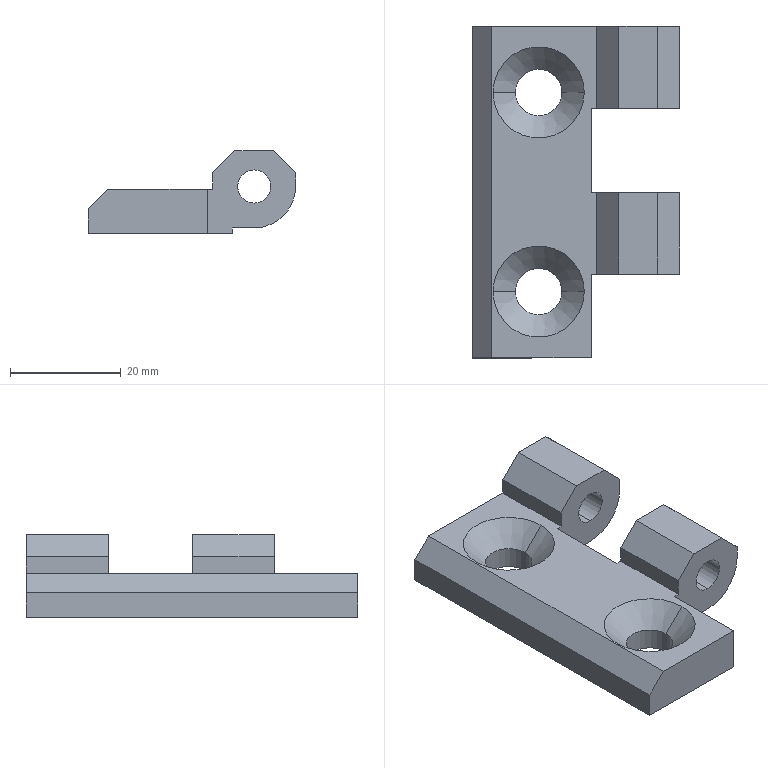Part | SolidWorks | features BaseBody 1 | 1 solid | 39 faces | box 37.5 x 60 x 15 mm | volume 13374 mm3 | plane 25 | cylinder 10 | cone 4 | commonest cylinder face diameters 6 x4 8.4 x4 15 x2
STEP:
#1=CARTESIAN_POINT('',(-13.8,-18.,0.));
#2=VERTEX_POINT('',#1);
#3=CARTESIAN_POINT('',(-22.2,-18.,0.));
#4=VERTEX_POINT('',#3);
#5=CARTESIAN_POINT('',(-18.,-18.,0.));
#6=DIRECTION('',(0.,0.,-1.));
#7=DIRECTION('',(1.,0.,0.));
#8=AXIS2_PLACEMENT_3D('',#5,#6,#7);
#9=CIRCLE('',#8,4.2);
#10=EDGE_CURVE('',#2,#4,#9,.T.);
#11=ORIENTED_EDGE('',*,*,#10,.T.);
#12=CARTESIAN_POINT('',(-22.2,-18.,3.95));
#13=VERTEX_POINT('',#12);
#14=CARTESIAN_POINT('',(-22.2,-18.,0.));
#15=DIRECTION('',(0.,0.,1.));
#16=VECTOR('',#15,1000.);
#17=LINE('',#14,#16);
#18=EDGE_CURVE('',#4,#13,#17,.T.);
#19=ORIENTED_EDGE('',*,*,#18,.T.);
#20=CARTESIAN_POINT('',(-13.8,-18.,3.95));
#21=VERTEX_POINT('',#20);
#22=CARTESIAN_POINT('',(-18.,-18.,3.95));
#23=DIRECTION('',(0.,0.,-1.));
#24=DIRECTION('',(1.,0.,0.));
#25=AXIS2_PLACEMENT_3D('',#22,#23,#24);
#26=CIRCLE('',#25,4.2);
#27=EDGE_CURVE('',#21,#13,#26,.T.);
#28=ORIENTED_EDGE('',*,*,#27,.F.);
#29=CARTESIAN_POINT('',(-13.8,-18.,0.));
#30=DIRECTION('',(0.,0.,1.));
#31=VECTOR('',#30,1000.);
#32=LINE('',#29,#31);
#33=EDGE_CURVE('',#2,#21,#32,.T.);
#34=ORIENTED_EDGE('',*,*,#33,.F.);
#35=EDGE_LOOP('',(#11,#19,#28,#34));
#36=FACE_OUTER_BOUND('',#35,.T.);
#37=CARTESIAN_POINT('',(-18.,-18.,0.));
#38=DIRECTION('',(0.,0.,1.));
#39=DIRECTION('',(1.,0.,0.));
#40=AXIS2_PLACEMENT_3D('',#37,#38,#39);
#41=CYLINDRICAL_SURFACE('',#40,4.2);
#42=ADVANCED_FACE('',(#36),#41,.F.);
#43=CARTESIAN_POINT('',(-13.8,18.,0.));
#44=VERTEX_POINT('',#43);
#45=CARTESIAN_POINT('',(-22.2,18.,0.));
#46=VERTEX_POINT('',#45);
#47=CARTESIAN_POINT('',(-18.,18.,0.));
#48=DIRECTION('',(0.,0.,-1.));
#49=DIRECTION('',(1.,0.,0.));
#50=AXIS2_PLACEMENT_3D('',#47,#48,#49);
#51=CIRCLE('',#50,4.2);
#52=EDGE_CURVE('',#44,#46,#51,.T.);
#53=ORIENTED_EDGE('',*,*,#52,.T.);
#54=CARTESIAN_POINT('',(-22.2,18.,3.95));
#55=VERTEX_POINT('',#54);
#56=CARTESIAN_POINT('',(-22.2,18.,0.));
#57=DIRECTION('',(0.,0.,1.));
#58=VECTOR('',#57,1000.);
#59=LINE('',#56,#58);
#60=EDGE_CURVE('',#46,#55,#59,.T.);
#61=ORIENTED_EDGE('',*,*,#60,.T.);
#62=CARTESIAN_POINT('',(-13.8,18.,3.95));
#63=VERTEX_POINT('',#62);
#64=CARTESIAN_POINT('',(-18.,18.,3.95));
#65=DIRECTION('',(0.,0.,-1.));
#66=DIRECTION('',(1.,0.,0.));
#67=AXIS2_PLACEMENT_3D('',#64,#65,#66);
#68=CIRCLE('',#67,4.2);
#69=EDGE_CURVE('',#63,#55,#68,.T.);
#70=ORIENTED_EDGE('',*,*,#69,.F.);
#71=CARTESIAN_POINT('',(-13.8,18.,0.));
#72=DIRECTION('',(0.,0.,1.));
#73=VECTOR('',#72,1000.);
#74=LINE('',#71,#73);
#75=EDGE_CURVE('',#44,#63,#74,.T.);
#76=ORIENTED_EDGE('',*,*,#75,.F.);
#77=EDGE_LOOP('',(#53,#61,#70,#76));
#78=FACE_OUTER_BOUND('',#77,.T.);
#79=CARTESIAN_POINT('',(-18.,18.,0.));
#80=DIRECTION('',(0.,0.,1.));
#81=DIRECTION('',(1.,0.,0.));
#82=AXIS2_PLACEMENT_3D('',#79,#80,#81);
#83=CYLINDRICAL_SURFACE('',#82,4.2);
#84=ADVANCED_FACE('',(#78),#83,.F.);
#85=ORIENTED_EDGE('',*,*,#27,.T.);
#86=CARTESIAN_POINT('',(-26.25,-18.,8.));
#87=VERTEX_POINT('',#86);
#88=CARTESIAN_POINT('',(-26.25,-18.,8.));
#89=DIRECTION('',(-0.7071,0.,0.7071));
#90=VECTOR('',#89,1000.);
#91=LINE('',#88,#90);
#92=EDGE_CURVE('',#13,#87,#91,.T.);
#93=ORIENTED_EDGE('',*,*,#92,.T.);
#94=CARTESIAN_POINT('',(-9.75,-18.,8.));
#95=VERTEX_POINT('',#94);
#96=CARTESIAN_POINT('',(-18.,-18.,8.));
#97=DIRECTION('',(0.,0.,-1.));
#98=DIRECTION('',(1.,0.,0.));
#99=AXIS2_PLACEMENT_3D('',#96,#97,#98);
#100=CIRCLE('',#99,8.25);
#101=EDGE_CURVE('',#95,#87,#100,.T.);
#102=ORIENTED_EDGE('',*,*,#101,.F.);
#103=CARTESIAN_POINT('',(-9.75,-18.,8.));
#104=DIRECTION('',(0.7071,0.,0.7071));
#105=VECTOR('',#104,1000.);
#106=LINE('',#103,#105);
#107=EDGE_CURVE('',#21,#95,#106,.T.);
#108=ORIENTED_EDGE('',*,*,#107,.F.);
#109=EDGE_LOOP('',(#85,#93,#102,#108));
#110=FACE_OUTER_BOUND('',#109,.T.);
#111=CARTESIAN_POINT('',(-18.,-18.,8.));
#112=DIRECTION('',(0.,0.,1.));
#113=DIRECTION('',(1.,0.,0.));
#114=AXIS2_PLACEMENT_3D('',#111,#112,#113);
#115=CONICAL_SURFACE('',#114,8.25,0.7854);
#116=ADVANCED_FACE('',(#110),#115,.F.);
#117=ORIENTED_EDGE('',*,*,#69,.T.);
#118=CARTESIAN_POINT('',(-26.25,18.,8.));
#119=VERTEX_POINT('',#118);
#120=CARTESIAN_POINT('',(-26.25,18.,8.));
#121=DIRECTION('',(-0.7071,0.,0.7071));
#122=VECTOR('',#121,1000.);
#123=LINE('',#120,#122);
#124=EDGE_CURVE('',#55,#119,#123,.T.);
#125=ORIENTED_EDGE('',*,*,#124,.T.);
#126=CARTESIAN_POINT('',(-9.75,18.,8.));
#127=VERTEX_POINT('',#126);
#128=CARTESIAN_POINT('',(-18.,18.,8.));
#129=DIRECTION('',(0.,0.,-1.));
#130=DIRECTION('',(1.,0.,0.));
#131=AXIS2_PLACEMENT_3D('',#128,#129,#130);
#132=CIRCLE('',#131,8.25);
#133=EDGE_CURVE('',#127,#119,#132,.T.);
#134=ORIENTED_EDGE('',*,*,#133,.F.);
#135=CARTESIAN_POINT('',(-9.75,18.,8.));
#136=DIRECTION('',(0.7071,0.,0.7071));
#137=VECTOR('',#136,1000.);
#138=LINE('',#135,#137);
#139=EDGE_CURVE('',#63,#127,#138,.T.);
#140=ORIENTED_EDGE('',*,*,#139,.F.);
#141=EDGE_LOOP('',(#117,#125,#134,#140));
#142=FACE_OUTER_BOUND('',#141,.T.);
#143=CARTESIAN_POINT('',(-18.,18.,8.));
#144=DIRECTION('',(0.,0.,1.));
#145=DIRECTION('',(1.,0.,0.));
#146=AXIS2_PLACEMENT_3D('',#143,#144,#145);
#147=CONICAL_SURFACE('',#146,8.25,0.7854);
#148=ADVANCED_FACE('',(#142),#147,.F.);
#149=CARTESIAN_POINT('',(0.,-14.85,5.5));
#150=VERTEX_POINT('',#149);
#151=CARTESIAN_POINT('',(0.,-14.85,11.5));
#152=VERTEX_POINT('',#151);
#153=CARTESIAN_POINT('',(0.,-14.85,8.5));
#154=DIRECTION('',(0.,1.,0.));
#155=DIRECTION('',(0.,0.,1.));
#156=AXIS2_PLACEMENT_3D('',#153,#154,#155);
#157=CIRCLE('',#156,3.);
#158=EDGE_CURVE('',#150,#152,#157,.T.);
#159=ORIENTED_EDGE('',*,*,#158,.F.);
#160=CARTESIAN_POINT('',(0.,-0.15,5.5));
#161=VERTEX_POINT('',#160);
#162=CARTESIAN_POINT('',(0.,-30.,5.5));
#163=DIRECTION('',(0.,1.,0.));
#164=VECTOR('',#163,1000.);
#165=LINE('',#162,#164);
#166=EDGE_CURVE('',#150,#161,#165,.T.);
#167=ORIENTED_EDGE('',*,*,#166,.T.);
#168=CARTESIAN_POINT('',(0.,-0.15,11.5));
#169=VERTEX_POINT('',#168);
#170=CARTESIAN_POINT('',(0.,-0.15,8.5));
#171=DIRECTION('',(0.,-1.,0.));
#172=DIRECTION('',(0.,0.,1.));
#173=AXIS2_PLACEMENT_3D('',#170,#171,#172);
#174=CIRCLE('',#173,3.);
#175=EDGE_CURVE('',#169,#161,#174,.T.);
#176=ORIENTED_EDGE('',*,*,#175,.F.);
#177=CARTESIAN_POINT('',(0.,-30.,11.5));
#178=DIRECTION('',(0.,1.,0.));
#179=VECTOR('',#178,1000.);
#180=LINE('',#177,#179);
#181=EDGE_CURVE('',#152,#169,#180,.T.);
#182=ORIENTED_EDGE('',*,*,#181,.F.);
#183=EDGE_LOOP('',(#159,#167,#176,#182));
#184=FACE_OUTER_BOUND('',#183,.T.);
#185=CARTESIAN_POINT('',(0.,-30.,8.5));
#186=DIRECTION('',(0.,1.,0.));
#187=DIRECTION('',(0.,0.,1.));
#188=AXIS2_PLACEMENT_3D('',#185,#186,#187);
#189=CYLINDRICAL_SURFACE('',#188,3.);
#190=ADVANCED_FACE('',(#184),#189,.F.);
#191=CARTESIAN_POINT('',(0.,15.15,5.5));
#192=VERTEX_POINT('',#191);
#193=CARTESIAN_POINT('',(0.,15.15,11.5));
#194=VERTEX_POINT('',#193);
#195=CARTESIAN_POINT('',(0.,15.15,8.5));
#196=DIRECTION('',(0.,1.,0.));
#197=DIRECTION('',(0.,0.,1.));
#198=AXIS2_PLACEMENT_3D('',#195,#196,#197);
#199=CIRCLE('',#198,3.);
#200=EDGE_CURVE('',#192,#194,#199,.T.);
#201=ORIENTED_EDGE('',*,*,#200,.F.);
#202=CARTESIAN_POINT('',(0.,30.,5.5));
#203=VERTEX_POINT('',#202);
#204=CARTESIAN_POINT('',(0.,-30.,5.5));
#205=DIRECTION('',(0.,1.,0.));
#206=VECTOR('',#205,1000.);
#207=LINE('',#204,#206);
#208=EDGE_CURVE('',#192,#203,#207,.T.);
#209=ORIENTED_EDGE('',*,*,#208,.T.);
#210=CARTESIAN_POINT('',(0.,30.,11.5));
#211=VERTEX_POINT('',#210);
#212=CARTESIAN_POINT('',(0.,30.,8.5));
#213=DIRECTION('',(0.,-1.,0.));
#214=DIRECTION('',(0.,0.,1.));
#215=AXIS2_PLACEMENT_3D('',#212,#213,#214);
#216=CIRCLE('',#215,3.);
#217=EDGE_CURVE('',#211,#203,#216,.T.);
#218=ORIENTED_EDGE('',*,*,#217,.F.);
#219=CARTESIAN_POINT('',(0.,-30.,11.5));
#220=DIRECTION('',(0.,1.,0.));
#221=VECTOR('',#220,1000.);
#222=LINE('',#219,#221);
#223=EDGE_CURVE('',#194,#211,#222,.T.);
#224=ORIENTED_EDGE('',*,*,#223,.F.);
#225=EDGE_LOOP('',(#201,#209,#218,#224));
#226=FACE_OUTER_BOUND('',#225,.T.);
#227=CARTESIAN_POINT('',(0.,-30.,8.5));
#228=DIRECTION('',(0.,1.,0.));
#229=DIRECTION('',(0.,0.,1.));
#230=AXIS2_PLACEMENT_3D('',#227,#228,#229);
#231=CYLINDRICAL_SURFACE('',#230,3.);
#232=ADVANCED_FACE('',(#226),#231,.F.);
#233=ORIENTED_EDGE('',*,*,#10,.F.);
#234=CARTESIAN_POINT('',(-18.,-18.,0.));
#235=DIRECTION('',(0.,0.,-1.));
#236=DIRECTION('',(1.,0.,0.));
#237=AXIS2_PLACEMENT_3D('',#234,#235,#236);
#238=CIRCLE('',#237,4.2);
#239=EDGE_CURVE('',#4,#2,#238,.T.);
#240=ORIENTED_EDGE('',*,*,#239,.F.);
#241=EDGE_LOOP('',(#233,#240));
#242=FACE_BOUND('',#241,.T.);
#243=ORIENTED_EDGE('',*,*,#52,.F.);
#244=CARTESIAN_POINT('',(-18.,18.,0.));
#245=DIRECTION('',(0.,0.,-1.));
#246=DIRECTION('',(1.,0.,0.));
#247=AXIS2_PLACEMENT_3D('',#244,#245,#246);
#248=CIRCLE('',#247,4.2);
#249=EDGE_CURVE('',#46,#44,#248,.T.);
#250=ORIENTED_EDGE('',*,*,#249,.F.);
#251=EDGE_LOOP('',(#243,#250));
#252=FACE_BOUND('',#251,.T.);
#253=CARTESIAN_POINT('',(-8.5,-14.85,0.));
#254=VERTEX_POINT('',#253);
#255=CARTESIAN_POINT('',(-4.,-14.85,0.));
#256=VERTEX_POINT('',#255);
#257=CARTESIAN_POINT('',(-4.,-14.85,0.));
#258=DIRECTION('',(1.,0.,0.));
#259=VECTOR('',#258,1000.);
#260=LINE('',#257,#259);
#261=EDGE_CURVE('',#254,#256,#260,.T.);
#262=ORIENTED_EDGE('',*,*,#261,.F.);
#263=CARTESIAN_POINT('',(-8.5,-30.,0.));
#264=VERTEX_POINT('',#263);
#265=CARTESIAN_POINT('',(-8.5,30.,0.));
#266=DIRECTION('',(0.,1.,0.));
#267=VECTOR('',#266,1000.);
#268=LINE('',#265,#267);
#269=EDGE_CURVE('',#264,#254,#268,.T.);
#270=ORIENTED_EDGE('',*,*,#269,.F.);
#271=CARTESIAN_POINT('',(-30.,-30.,0.));
#272=VERTEX_POINT('',#271);
#273=CARTESIAN_POINT('',(-4.,-30.,0.));
#274=DIRECTION('',(1.,0.,0.));
#275=VECTOR('',#274,1000.);
#276=LINE('',#273,#275);
#277=EDGE_CURVE('',#272,#264,#276,.T.);
#278=ORIENTED_EDGE('',*,*,#277,.F.);
#279=CARTESIAN_POINT('',(-30.,30.,0.));
#280=VERTEX_POINT('',#279);
#281=CARTESIAN_POINT('',(-30.,30.,0.));
#282=DIRECTION('',(0.,-1.,0.));
#283=VECTOR('',#282,1000.);
#284=LINE('',#281,#283);
#285=EDGE_CURVE('',#280,#272,#284,.T.);
#286=ORIENTED_EDGE('',*,*,#285,.F.);
#287=CARTESIAN_POINT('',(-4.,30.,0.));
#288=VERTEX_POINT('',#287);
#289=CARTESIAN_POINT('',(-4.,30.,0.));
#290=DIRECTION('',(-1.,0.,0.));
#291=VECTOR('',#290,1000.);
#292=LINE('',#289,#291);
#293=EDGE_CURVE('',#288,#280,#292,.T.);
#294=ORIENTED_EDGE('',*,*,#293,.F.);
#295=CARTESIAN_POINT('',(-4.,15.15,0.));
#296=VERTEX_POINT('',#295);
#297=CARTESIAN_POINT('',(-4.,30.,0.));
#298=DIRECTION('',(0.,1.,0.));
#299=VECTOR('',#298,1000.);
#300=LINE('',#297,#299);
#301=EDGE_CURVE('',#296,#288,#300,.T.);
#302=ORIENTED_EDGE('',*,*,#301,.F.);
#303=CARTESIAN_POINT('',(-8.5,15.15,0.));
#304=VERTEX_POINT('',#303);
#305=CARTESIAN_POINT('',(-4.,15.15,0.));
#306=DIRECTION('',(1.,0.,0.));
#307=VECTOR('',#306,1000.);
#308=LINE('',#305,#307);
#309=EDGE_CURVE('',#304,#296,#308,.T.);
#310=ORIENTED_EDGE('',*,*,#309,.F.);
#311=CARTESIAN_POINT('',(-8.5,-0.15,0.));
#312=VERTEX_POINT('',#311);
#313=CARTESIAN_POINT('',(-8.5,30.,0.));
#314=DIRECTION('',(0.,1.,0.));
#315=VECTOR('',#314,1000.);
#316=LINE('',#313,#315);
#317=EDGE_CURVE('',#312,#304,#316,.T.);
#318=ORIENTED_EDGE('',*,*,#317,.F.);
#319=CARTESIAN_POINT('',(-4.,-0.15,0.));
#320=VERTEX_POINT('',#319);
#321=CARTESIAN_POINT('',(-4.,-0.15,0.));
#322=DIRECTION('',(-1.,0.,0.));
#323=VECTOR('',#322,1000.);
#324=LINE('',#321,#323);
#325=EDGE_CURVE('',#320,#312,#324,.T.);
#326=ORIENTED_EDGE('',*,*,#325,.F.);
#327=CARTESIAN_POINT('',(-4.,30.,0.));
#328=DIRECTION('',(0.,1.,0.));
#329=VECTOR('',#328,1000.);
#330=LINE('',#327,#329);
#331=EDGE_CURVE('',#256,#320,#330,.T.);
#332=ORIENTED_EDGE('',*,*,#331,.F.);
#333=EDGE_LOOP('',(#262,#270,#278,#286,#294,#302,#310,#318,#326,#332));
#334=FACE_OUTER_BOUND('',#333,.T.);
#335=CARTESIAN_POINT('',(-4.,30.,0.));
#336=DIRECTION('',(0.,0.,1.));
#337=DIRECTION('',(1.,0.,0.));
#338=AXIS2_PLACEMENT_3D('',#335,#336,#337);
#339=PLANE('',#338);
#340=ADVANCED_FACE('',(#242,#252,#334),#339,.F.);
#341=ORIENTED_EDGE('',*,*,#18,.F.);
#342=ORIENTED_EDGE('',*,*,#239,.T.);
#343=ORIENTED_EDGE('',*,*,#33,.T.);
#344=CARTESIAN_POINT('',(-18.,-18.,3.95));
#345=DIRECTION('',(0.,0.,-1.));
#346=DIRECTION('',(1.,0.,0.));
#347=AXIS2_PLACEMENT_3D('',#344,#345,#346);
#348=CIRCLE('',#347,4.2);
#349=EDGE_CURVE('',#13,#21,#348,.T.);
#350=ORIENTED_EDGE('',*,*,#349,.F.);
#351=EDGE_LOOP('',(#341,#342,#343,#350));
#352=FACE_OUTER_BOUND('',#351,.T.);
#353=CARTESIAN_POINT('',(-18.,-18.,0.));
#354=DIRECTION('',(0.,0.,1.));
#355=DIRECTION('',(1.,0.,0.));
#356=AXIS2_PLACEMENT_3D('',#353,#354,#355);
#357=CYLINDRICAL_SURFACE('',#356,4.2);
#358=ADVANCED_FACE('',(#352),#357,.F.);
#359=ORIENTED_EDGE('',*,*,#60,.F.);
#360=ORIENTED_EDGE('',*,*,#249,.T.);
#361=ORIENTED_EDGE('',*,*,#75,.T.);
#362=CARTESIAN_POINT('',(-18.,18.,3.95));
#363=DIRECTION('',(0.,0.,-1.));
#364=DIRECTION('',(1.,0.,0.));
#365=AXIS2_PLACEMENT_3D('',#362,#363,#364);
#366=CIRCLE('',#365,4.2);
#367=EDGE_CURVE('',#55,#63,#366,.T.);
#368=ORIENTED_EDGE('',*,*,#367,.F.);
#369=EDGE_LOOP('',(#359,#360,#361,#368));
#370=FACE_OUTER_BOUND('',#369,.T.);
#371=CARTESIAN_POINT('',(-18.,18.,0.));
#372=DIRECTION('',(0.,0.,1.));
#373=DIRECTION('',(1.,0.,0.));
#374=AXIS2_PLACEMENT_3D('',#371,#372,#373);
#375=CYLINDRICAL_SURFACE('',#374,4.2);
#376=ADVANCED_FACE('',(#370),#375,.F.);
#377=CARTESIAN_POINT('',(-4.,-14.85,1.));
#378=VERTEX_POINT('',#377);
#379=CARTESIAN_POINT('',(-4.,-14.85,1.));
#380=DIRECTION('',(0.,0.,1.));
#381=VECTOR('',#380,1000.);
#382=LINE('',#379,#381);
#383=EDGE_CURVE('',#256,#378,#382,.T.);
#384=ORIENTED_EDGE('',*,*,#383,.F.);
#385=ORIENTED_EDGE('',*,*,#331,.T.);
#386=CARTESIAN_POINT('',(-4.,-0.15,1.));
#387=VERTEX_POINT('',#386);
#388=CARTESIAN_POINT('',(-4.,-0.15,1.));
#389=DIRECTION('',(0.,0.,-1.));
#390=VECTOR('',#389,1000.);
#391=LINE('',#388,#390);
#392=EDGE_CURVE('',#387,#320,#391,.T.);
#393=ORIENTED_EDGE('',*,*,#392,.F.);
#394=CARTESIAN_POINT('',(-4.,30.,1.));
#395=DIRECTION('',(0.,1.,0.));
#396=VECTOR('',#395,1000.);
#397=LINE('',#394,#396);
#398=EDGE_CURVE('',#378,#387,#397,.T.);
#399=ORIENTED_EDGE('',*,*,#398,.F.);
#400=EDGE_LOOP('',(#384,#385,#393,#399));
#401=FACE_OUTER_BOUND('',#400,.T.);
#402=CARTESIAN_POINT('',(-4.,30.,1.));
#403=DIRECTION('',(-1.,0.,0.));
#404=DIRECTION('',(0.,0.,1.));
#405=AXIS2_PLACEMENT_3D('',#402,#403,#404);
#406=PLANE('',#405);
#407=ADVANCED_FACE('',(#401),#406,.F.);
#408=CARTESIAN_POINT('',(0.,-14.85,8.5));
#409=DIRECTION('',(0.,1.,0.));
#410=DIRECTION('',(0.,0.,1.));
#411=AXIS2_PLACEMENT_3D('',#408,#409,#410);
#412=CIRCLE('',#411,3.);
#413=EDGE_CURVE('',#152,#150,#412,.T.);
#414=ORIENTED_EDGE('',*,*,#413,.T.);
#415=ORIENTED_EDGE('',*,*,#158,.T.);
#416=EDGE_LOOP('',(#414,#415));
#417=FACE_BOUND('',#416,.T.);
#418=CARTESIAN_POINT('',(7.5,-14.85,11.));
#419=VERTEX_POINT('',#418);
#420=CARTESIAN_POINT('',(3.5,-14.85,15.));
#421=VERTEX_POINT('',#420);
#422=CARTESIAN_POINT('',(7.5,-14.85,11.));
#423=DIRECTION('',(-0.7071,0.,0.7071));
#424=VECTOR('',#423,1000.);
#425=LINE('',#422,#424);
#426=EDGE_CURVE('',#419,#421,#425,.T.);
#427=ORIENTED_EDGE('',*,*,#426,.T.);
#428=CARTESIAN_POINT('',(-3.5,-14.85,15.));
#429=VERTEX_POINT('',#428);
#430=CARTESIAN_POINT('',(8.5,-14.85,15.));
#431=DIRECTION('',(-1.,0.,0.));
#432=VECTOR('',#431,1000.);
#433=LINE('',#430,#432);
#434=EDGE_CURVE('',#421,#429,#433,.T.);
#435=ORIENTED_EDGE('',*,*,#434,.T.);
#436=CARTESIAN_POINT('',(-7.5,-14.85,11.));
#437=VERTEX_POINT('',#436);
#438=CARTESIAN_POINT('',(-3.5,-14.85,15.));
#439=DIRECTION('',(-0.7071,0.,-0.7071));
#440=VECTOR('',#439,1000.);
#441=LINE('',#438,#440);
#442=EDGE_CURVE('',#429,#437,#441,.T.);
#443=ORIENTED_EDGE('',*,*,#442,.T.);
#444=CARTESIAN_POINT('',(-7.5,-14.85,8.));
#445=VERTEX_POINT('',#444);
#446=CARTESIAN_POINT('',(-7.5,-14.85,15.));
#447=DIRECTION('',(0.,0.,-1.));
#448=VECTOR('',#447,1000.);
#449=LINE('',#446,#448);
#450=EDGE_CURVE('',#437,#445,#449,.T.);
#451=ORIENTED_EDGE('',*,*,#450,.T.);
#452=CARTESIAN_POINT('',(-8.5,-14.85,8.));
#453=VERTEX_POINT('',#452);
#454=CARTESIAN_POINT('',(-26.5,-14.85,8.));
#455=DIRECTION('',(-1.,0.,0.));
#456=VECTOR('',#455,1000.);
#457=LINE('',#454,#456);
#458=EDGE_CURVE('',#445,#453,#457,.T.);
#459=ORIENTED_EDGE('',*,*,#458,.T.);
#460=CARTESIAN_POINT('',(-8.5,-14.85,15.));
#461=DIRECTION('',(0.,0.,-1.));
#462=VECTOR('',#461,1000.);
#463=LINE('',#460,#462);
#464=EDGE_CURVE('',#453,#254,#463,.T.);
#465=ORIENTED_EDGE('',*,*,#464,.T.);
#466=ORIENTED_EDGE('',*,*,#261,.T.);
#467=ORIENTED_EDGE('',*,*,#383,.T.);
#468=CARTESIAN_POINT('',(0.,-14.85,1.));
#469=VERTEX_POINT('',#468);
#470=CARTESIAN_POINT('',(8.5,-14.85,1.));
#471=DIRECTION('',(1.,0.,0.));
#472=VECTOR('',#471,1000.);
#473=LINE('',#470,#472);
#474=EDGE_CURVE('',#378,#469,#473,.T.);
#475=ORIENTED_EDGE('',*,*,#474,.T.);
#476=CARTESIAN_POINT('',(7.5,-14.85,8.5));
#477=VERTEX_POINT('',#476);
#478=CARTESIAN_POINT('',(0.,-14.85,8.5));
#479=DIRECTION('',(0.,-1.,0.));
#480=DIRECTION('',(0.,0.,1.));
#481=AXIS2_PLACEMENT_3D('',#478,#479,#480);
#482=CIRCLE('',#481,7.5);
#483=EDGE_CURVE('',#469,#477,#482,.T.);
#484=ORIENTED_EDGE('',*,*,#483,.T.);
#485=CARTESIAN_POINT('',(7.5,-14.85,15.));
#486=DIRECTION('',(0.,0.,1.));
#487=VECTOR('',#486,1000.);
#488=LINE('',#485,#487);
#489=EDGE_CURVE('',#477,#419,#488,.T.);
#490=ORIENTED_EDGE('',*,*,#489,.T.);
#491=EDGE_LOOP('',(#427,#435,#443,#451,#459,#465,#466,#467,#475,#484,#490));
#492=FACE_OUTER_BOUND('',#491,.T.);
#493=CARTESIAN_POINT('',(8.5,-14.85,15.));
#494=DIRECTION('',(0.,-1.,0.));
#495=DIRECTION('',(0.,0.,-1.));
#496=AXIS2_PLACEMENT_3D('',#493,#494,#495);
#497=PLANE('',#496);
#498=ADVANCED_FACE('',(#417,#492),#497,.T.);
#499=CARTESIAN_POINT('',(-8.5,-30.,8.));
#500=VERTEX_POINT('',#499);
#501=CARTESIAN_POINT('',(-8.5,-14.85,8.));
#502=DIRECTION('',(0.,-1.,0.));
#503=VECTOR('',#502,1000.);
#504=LINE('',#501,#503);
#505=EDGE_CURVE('',#453,#500,#504,.T.);
#506=ORIENTED_EDGE('',*,*,#505,.T.);
#507=CARTESIAN_POINT('',(-8.5,-30.,15.));
#508=DIRECTION('',(0.,0.,-1.));
#509=VECTOR('',#508,1000.);
#510=LINE('',#507,#509);
#511=EDGE_CURVE('',#500,#264,#510,.T.);
#512=ORIENTED_EDGE('',*,*,#511,.T.);
#513=ORIENTED_EDGE('',*,*,#269,.T.);
#514=ORIENTED_EDGE('',*,*,#464,.F.);
#515=EDGE_LOOP('',(#506,#512,#513,#514));
#516=FACE_OUTER_BOUND('',#515,.T.);
#517=CARTESIAN_POINT('',(-8.5,-14.85,15.));
#518=DIRECTION('',(1.,0.,0.));
#519=DIRECTION('',(0.,0.,-1.));
#520=AXIS2_PLACEMENT_3D('',#517,#518,#519);
#521=PLANE('',#520);
#522=ADVANCED_FACE('',(#516),#521,.T.);
#523=CARTESIAN_POINT('',(-30.,-30.,4.5));
#524=VERTEX_POINT('',#523);
#525=CARTESIAN_POINT('',(-26.5,-30.,8.));
#526=VERTEX_POINT('',#525);
#527=CARTESIAN_POINT('',(-30.,-30.,4.5));
#528=DIRECTION('',(0.7071,0.,0.7071));
#529=VECTOR('',#528,1000.);
#530=LINE('',#527,#529);
#531=EDGE_CURVE('',#524,#526,#530,.T.);
#532=ORIENTED_EDGE('',*,*,#531,.F.);
#533=CARTESIAN_POINT('',(-30.,-30.,8.5));
#534=DIRECTION('',(0.,0.,1.));
#535=VECTOR('',#534,1000.);
#536=LINE('',#533,#535);
#537=EDGE_CURVE('',#272,#524,#536,.T.);
#538=ORIENTED_EDGE('',*,*,#537,.F.);
#539=ORIENTED_EDGE('',*,*,#277,.T.);
#540=ORIENTED_EDGE('',*,*,#511,.F.);
#541=CARTESIAN_POINT('',(0.,-30.,8.));
#542=DIRECTION('',(1.,0.,0.));
#543=VECTOR('',#542,1000.);
#544=LINE('',#541,#543);
#545=EDGE_CURVE('',#526,#500,#544,.T.);
#546=ORIENTED_EDGE('',*,*,#545,.F.);
#547=EDGE_LOOP('',(#532,#538,#539,#540,#546));
#548=FACE_OUTER_BOUND('',#547,.T.);
#549=CARTESIAN_POINT('',(0.,-30.,8.5));
#550=DIRECTION('',(0.,1.,0.));
#551=DIRECTION('',(0.,0.,1.));
#552=AXIS2_PLACEMENT_3D('',#549,#550,#551);
#553=PLANE('',#552);
#554=ADVANCED_FACE('',(#548),#553,.F.);
#555=CARTESIAN_POINT('',(-30.,30.,4.5));
#556=VERTEX_POINT('',#555);
#557=CARTESIAN_POINT('',(-30.,30.,0.));
#558=DIRECTION('',(0.,0.,1.));
#559=VECTOR('',#558,1000.);
#560=LINE('',#557,#559);
#561=EDGE_CURVE('',#280,#556,#560,.T.);
#562=ORIENTED_EDGE('',*,*,#561,.F.);
#563=ORIENTED_EDGE('',*,*,#285,.T.);
#564=ORIENTED_EDGE('',*,*,#537,.T.);
#565=CARTESIAN_POINT('',(-30.,30.,4.5));
#566=DIRECTION('',(0.,-1.,0.));
#567=VECTOR('',#566,1000.);
#568=LINE('',#565,#567);
#569=EDGE_CURVE('',#556,#524,#568,.T.);
#570=ORIENTED_EDGE('',*,*,#569,.F.);
#571=EDGE_LOOP('',(#562,#563,#564,#570));
#572=FACE_OUTER_BOUND('',#571,.T.);
#573=CARTESIAN_POINT('',(-30.,30.,0.));
#574=DIRECTION('',(1.,0.,0.));
#575=DIRECTION('',(0.,0.,-1.));
#576=AXIS2_PLACEMENT_3D('',#573,#574,#575);
#577=PLANE('',#576);
#578=ADVANCED_FACE('',(#572),#577,.F.);
#579=ORIENTED_EDGE('',*,*,#217,.T.);
#580=CARTESIAN_POINT('',(0.,30.,8.5));
#581=DIRECTION('',(0.,-1.,0.));
#582=DIRECTION('',(0.,0.,1.));
#583=AXIS2_PLACEMENT_3D('',#580,#581,#582);
#584=CIRCLE('',#583,3.);
#585=EDGE_CURVE('',#203,#211,#584,.T.);
#586=ORIENTED_EDGE('',*,*,#585,.T.);
#587=EDGE_LOOP('',(#579,#586));
#588=FACE_BOUND('',#587,.T.);
#589=CARTESIAN_POINT('',(7.5,30.,8.5));
#590=VERTEX_POINT('',#589);
#591=CARTESIAN_POINT('',(0.,30.,1.));
#592=VERTEX_POINT('',#591);
#593=CARTESIAN_POINT('',(0.,30.,8.5));
#594=DIRECTION('',(0.,1.,0.));
#595=DIRECTION('',(0.,0.,1.));
#596=AXIS2_PLACEMENT_3D('',#593,#594,#595);
#597=CIRCLE('',#596,7.5);
#598=EDGE_CURVE('',#590,#592,#597,.T.);
#599=ORIENTED_EDGE('',*,*,#598,.T.);
#600=CARTESIAN_POINT('',(-4.,30.,1.));
#601=VERTEX_POINT('',#600);
#602=CARTESIAN_POINT('',(0.,30.,1.));
#603=DIRECTION('',(-1.,0.,0.));
#604=VECTOR('',#603,1000.);
#605=LINE('',#602,#604);
#606=EDGE_CURVE('',#592,#601,#605,.T.);
#607=ORIENTED_EDGE('',*,*,#606,.T.);
#608=CARTESIAN_POINT('',(-4.,30.,8.5));
#609=DIRECTION('',(0.,0.,-1.));
#610=VECTOR('',#609,1000.);
#611=LINE('',#608,#610);
#612=EDGE_CURVE('',#601,#288,#611,.T.);
#613=ORIENTED_EDGE('',*,*,#612,.T.);
#614=ORIENTED_EDGE('',*,*,#293,.T.);
#615=ORIENTED_EDGE('',*,*,#561,.T.);
#616=CARTESIAN_POINT('',(-26.5,30.,8.));
#617=VERTEX_POINT('',#616);
#618=CARTESIAN_POINT('',(-30.,30.,4.5));
#619=DIRECTION('',(0.7071,0.,0.7071));
#620=VECTOR('',#619,1000.);
#621=LINE('',#618,#620);
#622=EDGE_CURVE('',#556,#617,#621,.T.);
#623=ORIENTED_EDGE('',*,*,#622,.T.);
#624=CARTESIAN_POINT('',(-7.5,30.,8.));
#625=VERTEX_POINT('',#624);
#626=CARTESIAN_POINT('',(0.,30.,8.));
#627=DIRECTION('',(1.,0.,0.));
#628=VECTOR('',#627,1000.);
#629=LINE('',#626,#628);
#630=EDGE_CURVE('',#617,#625,#629,.T.);
#631=ORIENTED_EDGE('',*,*,#630,.T.);
#632=CARTESIAN_POINT('',(-7.5,30.,11.));
#633=VERTEX_POINT('',#632);
#634=CARTESIAN_POINT('',(-7.5,30.,8.5));
#635=DIRECTION('',(0.,0.,1.));
#636=VECTOR('',#635,1000.);
#637=LINE('',#634,#636);
#638=EDGE_CURVE('',#625,#633,#637,.T.);
#639=ORIENTED_EDGE('',*,*,#638,.T.);
#640=CARTESIAN_POINT('',(-3.5,30.,15.));
#641=VERTEX_POINT('',#640);
#642=CARTESIAN_POINT('',(-7.5,30.,11.));
#643=DIRECTION('',(0.7071,0.,0.7071));
#644=VECTOR('',#643,1000.);
#645=LINE('',#642,#644);
#646=EDGE_CURVE('',#633,#641,#645,.T.);
#647=ORIENTED_EDGE('',*,*,#646,.T.);
#648=CARTESIAN_POINT('',(3.5,30.,15.));
#649=VERTEX_POINT('',#648);
#650=CARTESIAN_POINT('',(0.,30.,15.));
#651=DIRECTION('',(1.,0.,0.));
#652=VECTOR('',#651,1000.);
#653=LINE('',#650,#652);
#654=EDGE_CURVE('',#641,#649,#653,.T.);
#655=ORIENTED_EDGE('',*,*,#654,.T.);
#656=CARTESIAN_POINT('',(7.5,30.,11.));
#657=VERTEX_POINT('',#656);
#658=CARTESIAN_POINT('',(3.5,30.,15.));
#659=DIRECTION('',(0.7071,0.,-0.7071));
#660=VECTOR('',#659,1000.);
#661=LINE('',#658,#660);
#662=EDGE_CURVE('',#649,#657,#661,.T.);
#663=ORIENTED_EDGE('',*,*,#662,.T.);
#664=CARTESIAN_POINT('',(7.5,30.,8.5));
#665=DIRECTION('',(0.,0.,-1.));
#666=VECTOR('',#665,1000.);
#667=LINE('',#664,#666);
#668=EDGE_CURVE('',#657,#590,#667,.T.);
#669=ORIENTED_EDGE('',*,*,#668,.T.);
#670=EDGE_LOOP('',(#599,#607,#613,#614,#615,#623,#631,#639,#647,#655,#663,#669));
#671=FACE_OUTER_BOUND('',#670,.T.);
#672=CARTESIAN_POINT('',(0.,30.,8.5));
#673=DIRECTION('',(0.,1.,0.));
#674=DIRECTION('',(0.,0.,1.));
#675=AXIS2_PLACEMENT_3D('',#672,#673,#674);
#676=PLANE('',#675);
#677=ADVANCED_FACE('',(#588,#671),#676,.T.);
#678=ORIENTED_EDGE('',*,*,#612,.F.);
#679=CARTESIAN_POINT('',(-4.,15.15,1.));
#680=VERTEX_POINT('',#679);
#681=CARTESIAN_POINT('',(-4.,30.,1.));
#682=DIRECTION('',(0.,1.,0.));
#683=VECTOR('',#682,1000.);
#684=LINE('',#681,#683);
#685=EDGE_CURVE('',#680,#601,#684,.T.);
#686=ORIENTED_EDGE('',*,*,#685,.F.);
#687=CARTESIAN_POINT('',(-4.,15.15,1.));
#688=DIRECTION('',(0.,0.,1.));
#689=VECTOR('',#688,1000.);
#690=LINE('',#687,#689);
#691=EDGE_CURVE('',#296,#680,#690,.T.);
#692=ORIENTED_EDGE('',*,*,#691,.F.);
#693=ORIENTED_EDGE('',*,*,#301,.T.);
#694=EDGE_LOOP('',(#678,#686,#692,#693));
#695=FACE_OUTER_BOUND('',#694,.T.);
#696=CARTESIAN_POINT('',(-4.,30.,1.));
#697=DIRECTION('',(-1.,0.,0.));
#698=DIRECTION('',(0.,0.,1.));
#699=AXIS2_PLACEMENT_3D('',#696,#697,#698);
#700=PLANE('',#699);
#701=ADVANCED_FACE('',(#695),#700,.F.);
#702=CARTESIAN_POINT('',(0.,15.15,8.5));
#703=DIRECTION('',(0.,1.,0.));
#704=DIRECTION('',(0.,0.,1.));
#705=AXIS2_PLACEMENT_3D('',#702,#703,#704);
#706=CIRCLE('',#705,3.);
#707=EDGE_CURVE('',#194,#192,#706,.T.);
#708=ORIENTED_EDGE('',*,*,#707,.T.);
#709=ORIENTED_EDGE('',*,*,#200,.T.);
#710=EDGE_LOOP('',(#708,#709));
#711=FACE_BOUND('',#710,.T.);
#712=CARTESIAN_POINT('',(7.5,15.15,11.));
#713=VERTEX_POINT('',#712);
#714=CARTESIAN_POINT('',(3.5,15.15,15.));
#715=VERTEX_POINT('',#714);
#716=CARTESIAN_POINT('',(7.5,15.15,11.));
#717=DIRECTION('',(-0.7071,0.,0.7071));
#718=VECTOR('',#717,1000.);
#719=LINE('',#716,#718);
#720=EDGE_CURVE('',#713,#715,#719,.T.);
#721=ORIENTED_EDGE('',*,*,#720,.T.);
#722=CARTESIAN_POINT('',(-3.5,15.15,15.));
#723=VERTEX_POINT('',#722);
#724=CARTESIAN_POINT('',(8.5,15.15,15.));
#725=DIRECTION('',(-1.,0.,0.));
#726=VECTOR('',#725,1000.);
#727=LINE('',#724,#726);
#728=EDGE_CURVE('',#715,#723,#727,.T.);
#729=ORIENTED_EDGE('',*,*,#728,.T.);
#730=CARTESIAN_POINT('',(-7.5,15.15,11.));
#731=VERTEX_POINT('',#730);
#732=CARTESIAN_POINT('',(-3.5,15.15,15.));
#733=DIRECTION('',(-0.7071,0.,-0.7071));
#734=VECTOR('',#733,1000.);
#735=LINE('',#732,#734);
#736=EDGE_CURVE('',#723,#731,#735,.T.);
#737=ORIENTED_EDGE('',*,*,#736,.T.);
#738=CARTESIAN_POINT('',(-7.5,15.15,8.));
#739=VERTEX_POINT('',#738);
#740=CARTESIAN_POINT('',(-7.5,15.15,15.));
#741=DIRECTION('',(0.,0.,-1.));
#742=VECTOR('',#741,1000.);
#743=LINE('',#740,#742);
#744=EDGE_CURVE('',#731,#739,#743,.T.);
#745=ORIENTED_EDGE('',*,*,#744,.T.);
#746=CARTESIAN_POINT('',(-8.5,15.15,8.));
#747=VERTEX_POINT('',#746);
#748=CARTESIAN_POINT('',(8.5,15.15,8.));
#749=DIRECTION('',(-1.,0.,0.));
#750=VECTOR('',#749,1000.);
#751=LINE('',#748,#750);
#752=EDGE_CURVE('',#739,#747,#751,.T.);
#753=ORIENTED_EDGE('',*,*,#752,.T.);
#754=CARTESIAN_POINT('',(-8.5,15.15,15.));
#755=DIRECTION('',(0.,0.,-1.));
#756=VECTOR('',#755,1000.);
#757=LINE('',#754,#756);
#758=EDGE_CURVE('',#747,#304,#757,.T.);
#759=ORIENTED_EDGE('',*,*,#758,.T.);
#760=ORIENTED_EDGE('',*,*,#309,.T.);
#761=ORIENTED_EDGE('',*,*,#691,.T.);
#762=CARTESIAN_POINT('',(0.,15.15,1.));
#763=VERTEX_POINT('',#762);
#764=CARTESIAN_POINT('',(8.5,15.15,1.));
#765=DIRECTION('',(1.,0.,0.));
#766=VECTOR('',#765,1000.);
#767=LINE('',#764,#766);
#768=EDGE_CURVE('',#680,#763,#767,.T.);
#769=ORIENTED_EDGE('',*,*,#768,.T.);
#770=CARTESIAN_POINT('',(7.5,15.15,8.5));
#771=VERTEX_POINT('',#770);
#772=CARTESIAN_POINT('',(0.,15.15,8.5));
#773=DIRECTION('',(0.,-1.,0.));
#774=DIRECTION('',(0.,0.,1.));
#775=AXIS2_PLACEMENT_3D('',#772,#773,#774);
#776=CIRCLE('',#775,7.5);
#777=EDGE_CURVE('',#763,#771,#776,.T.);
#778=ORIENTED_EDGE('',*,*,#777,.T.);
#779=CARTESIAN_POINT('',(7.5,15.15,15.));
#780=DIRECTION('',(0.,0.,1.));
#781=VECTOR('',#780,1000.);
#782=LINE('',#779,#781);
#783=EDGE_CURVE('',#771,#713,#782,.T.);
#784=ORIENTED_EDGE('',*,*,#783,.T.);
#785=EDGE_LOOP('',(#721,#729,#737,#745,#753,#759,#760,#761,#769,#778,#784));
#786=FACE_OUTER_BOUND('',#785,.T.);
#787=CARTESIAN_POINT('',(8.5,15.15,15.));
#788=DIRECTION('',(0.,-1.,0.));
#789=DIRECTION('',(0.,0.,-1.));
#790=AXIS2_PLACEMENT_3D('',#787,#788,#789);
#791=PLANE('',#790);
#792=ADVANCED_FACE('',(#711,#786),#791,.T.);
#793=CARTESIAN_POINT('',(-8.5,-0.15,8.));
#794=VERTEX_POINT('',#793);
#795=CARTESIAN_POINT('',(-8.5,15.15,8.));
#796=DIRECTION('',(0.,-1.,0.));
#797=VECTOR('',#796,1000.);
#798=LINE('',#795,#797);
#799=EDGE_CURVE('',#747,#794,#798,.T.);
#800=ORIENTED_EDGE('',*,*,#799,.T.);
#801=CARTESIAN_POINT('',(-8.5,-0.15,15.));
#802=DIRECTION('',(0.,0.,-1.));
#803=VECTOR('',#802,1000.);
#804=LINE('',#801,#803);
#805=EDGE_CURVE('',#794,#312,#804,.T.);
#806=ORIENTED_EDGE('',*,*,#805,.T.);
#807=ORIENTED_EDGE('',*,*,#317,.T.);
#808=ORIENTED_EDGE('',*,*,#758,.F.);
#809=EDGE_LOOP('',(#800,#806,#807,#808));
#810=FACE_OUTER_BOUND('',#809,.T.);
#811=CARTESIAN_POINT('',(-8.5,15.15,15.));
#812=DIRECTION('',(1.,0.,0.));
#813=DIRECTION('',(0.,0.,-1.));
#814=AXIS2_PLACEMENT_3D('',#811,#812,#813);
#815=PLANE('',#814);
#816=ADVANCED_FACE('',(#810),#815,.T.);
#817=ORIENTED_EDGE('',*,*,#175,.T.);
#818=CARTESIAN_POINT('',(0.,-0.15,8.5));
#819=DIRECTION('',(0.,-1.,0.));
#820=DIRECTION('',(0.,0.,1.));
#821=AXIS2_PLACEMENT_3D('',#818,#819,#820);
#822=CIRCLE('',#821,3.);
#823=EDGE_CURVE('',#161,#169,#822,.T.);
#824=ORIENTED_EDGE('',*,*,#823,.T.);
#825=EDGE_LOOP('',(#817,#824));
#826=FACE_BOUND('',#825,.T.);
#827=CARTESIAN_POINT('',(0.,-0.15,1.));
#828=VERTEX_POINT('',#827);
#829=CARTESIAN_POINT('',(-8.5,-0.15,1.));
#830=DIRECTION('',(-1.,0.,0.));
#831=VECTOR('',#830,1000.);
#832=LINE('',#829,#831);
#833=EDGE_CURVE('',#828,#387,#832,.T.);
#834=ORIENTED_EDGE('',*,*,#833,.T.);
#835=ORIENTED_EDGE('',*,*,#392,.T.);
#836=ORIENTED_EDGE('',*,*,#325,.T.);
#837=ORIENTED_EDGE('',*,*,#805,.F.);
#838=CARTESIAN_POINT('',(-7.5,-0.15,8.));
#839=VERTEX_POINT('',#838);
#840=CARTESIAN_POINT('',(-8.5,-0.15,8.));
#841=DIRECTION('',(1.,0.,0.));
#842=VECTOR('',#841,1000.);
#843=LINE('',#840,#842);
#844=EDGE_CURVE('',#794,#839,#843,.T.);
#845=ORIENTED_EDGE('',*,*,#844,.T.);
#846=CARTESIAN_POINT('',(-7.5,-0.15,11.));
#847=VERTEX_POINT('',#846);
#848=CARTESIAN_POINT('',(-7.5,-0.15,15.));
#849=DIRECTION('',(0.,0.,1.));
#850=VECTOR('',#849,1000.);
#851=LINE('',#848,#850);
#852=EDGE_CURVE('',#839,#847,#851,.T.);
#853=ORIENTED_EDGE('',*,*,#852,.T.);
#854=CARTESIAN_POINT('',(-3.5,-0.15,15.));
#855=VERTEX_POINT('',#854);
#856=CARTESIAN_POINT('',(-7.5,-0.15,11.));
#857=DIRECTION('',(0.7071,0.,0.7071));
#858=VECTOR('',#857,1000.);
#859=LINE('',#856,#858);
#860=EDGE_CURVE('',#847,#855,#859,.T.);
#861=ORIENTED_EDGE('',*,*,#860,.T.);
#862=CARTESIAN_POINT('',(3.5,-0.15,15.));
#863=VERTEX_POINT('',#862);
#864=CARTESIAN_POINT('',(-8.5,-0.15,15.));
#865=DIRECTION('',(1.,0.,0.));
#866=VECTOR('',#865,1000.);
#867=LINE('',#864,#866);
#868=EDGE_CURVE('',#855,#863,#867,.T.);
#869=ORIENTED_EDGE('',*,*,#868,.T.);
#870=CARTESIAN_POINT('',(7.5,-0.15,11.));
#871=VERTEX_POINT('',#870);
#872=CARTESIAN_POINT('',(3.5,-0.15,15.));
#873=DIRECTION('',(0.7071,0.,-0.7071));
#874=VECTOR('',#873,1000.);
#875=LINE('',#872,#874);
#876=EDGE_CURVE('',#863,#871,#875,.T.);
#877=ORIENTED_EDGE('',*,*,#876,.T.);
#878=CARTESIAN_POINT('',(7.5,-0.15,8.5));
#879=VERTEX_POINT('',#878);
#880=CARTESIAN_POINT('',(7.5,-0.15,15.));
#881=DIRECTION('',(0.,0.,-1.));
#882=VECTOR('',#881,1000.);
#883=LINE('',#880,#882);
#884=EDGE_CURVE('',#871,#879,#883,.T.);
#885=ORIENTED_EDGE('',*,*,#884,.T.);
#886=CARTESIAN_POINT('',(0.,-0.15,8.5));
#887=DIRECTION('',(0.,1.,0.));
#888=DIRECTION('',(0.,0.,1.));
#889=AXIS2_PLACEMENT_3D('',#886,#887,#888);
#890=CIRCLE('',#889,7.5);
#891=EDGE_CURVE('',#879,#828,#890,.T.);
#892=ORIENTED_EDGE('',*,*,#891,.T.);
#893=EDGE_LOOP('',(#834,#835,#836,#837,#845,#853,#861,#869,#877,#885,#892));
#894=FACE_OUTER_BOUND('',#893,.T.);
#895=CARTESIAN_POINT('',(-8.5,-0.15,15.));
#896=DIRECTION('',(0.,1.,0.));
#897=DIRECTION('',(0.,0.,1.));
#898=AXIS2_PLACEMENT_3D('',#895,#896,#897);
#899=PLANE('',#898);
#900=ADVANCED_FACE('',(#826,#894),#899,.T.);
#901=ORIENTED_EDGE('',*,*,#92,.F.);
#902=ORIENTED_EDGE('',*,*,#349,.T.);
#903=ORIENTED_EDGE('',*,*,#107,.T.);
#904=CARTESIAN_POINT('',(-18.,-18.,8.));
#905=DIRECTION('',(0.,0.,-1.));
#906=DIRECTION('',(1.,0.,0.));
#907=AXIS2_PLACEMENT_3D('',#904,#905,#906);
#908=CIRCLE('',#907,8.25);
#909=EDGE_CURVE('',#87,#95,#908,.T.);
#910=ORIENTED_EDGE('',*,*,#909,.F.);
#911=EDGE_LOOP('',(#901,#902,#903,#910));
#912=FACE_OUTER_BOUND('',#911,.T.);
#913=CARTESIAN_POINT('',(-18.,-18.,8.));
#914=DIRECTION('',(0.,0.,1.));
#915=DIRECTION('',(1.,0.,0.));
#916=AXIS2_PLACEMENT_3D('',#913,#914,#915);
#917=CONICAL_SURFACE('',#916,8.25,0.7854);
#918=ADVANCED_FACE('',(#912),#917,.F.);
#919=ORIENTED_EDGE('',*,*,#124,.F.);
#920=ORIENTED_EDGE('',*,*,#367,.T.);
#921=ORIENTED_EDGE('',*,*,#139,.T.);
#922=CARTESIAN_POINT('',(-18.,18.,8.));
#923=DIRECTION('',(0.,0.,-1.));
#924=DIRECTION('',(1.,0.,0.));
#925=AXIS2_PLACEMENT_3D('',#922,#923,#924);
#926=CIRCLE('',#925,8.25);
#927=EDGE_CURVE('',#119,#127,#926,.T.);
#928=ORIENTED_EDGE('',*,*,#927,.F.);
#929=EDGE_LOOP('',(#919,#920,#921,#928));
#930=FACE_OUTER_BOUND('',#929,.T.);
#931=CARTESIAN_POINT('',(-18.,18.,8.));
#932=DIRECTION('',(0.,0.,1.));
#933=DIRECTION('',(1.,0.,0.));
#934=AXIS2_PLACEMENT_3D('',#931,#932,#933);
#935=CONICAL_SURFACE('',#934,8.25,0.7854);
#936=ADVANCED_FACE('',(#930),#935,.F.);
#937=ORIENTED_EDGE('',*,*,#474,.F.);
#938=ORIENTED_EDGE('',*,*,#398,.T.);
#939=ORIENTED_EDGE('',*,*,#833,.F.);
#940=CARTESIAN_POINT('',(0.,30.,1.));
#941=DIRECTION('',(0.,1.,0.));
#942=VECTOR('',#941,1000.);
#943=LINE('',#940,#942);
#944=EDGE_CURVE('',#469,#828,#943,.T.);
#945=ORIENTED_EDGE('',*,*,#944,.F.);
#946=EDGE_LOOP('',(#937,#938,#939,#945));
#947=FACE_OUTER_BOUND('',#946,.T.);
#948=CARTESIAN_POINT('',(0.,30.,1.));
#949=DIRECTION('',(0.,0.,1.));
#950=DIRECTION('',(1.,0.,0.));
#951=AXIS2_PLACEMENT_3D('',#948,#949,#950);
#952=PLANE('',#951);
#953=ADVANCED_FACE('',(#947),#952,.F.);
#954=ORIENTED_EDGE('',*,*,#166,.F.);
#955=ORIENTED_EDGE('',*,*,#413,.F.);
#956=ORIENTED_EDGE('',*,*,#181,.T.);
#957=ORIENTED_EDGE('',*,*,#823,.F.);
#958=EDGE_LOOP('',(#954,#955,#956,#957));
#959=FACE_OUTER_BOUND('',#958,.T.);
#960=CARTESIAN_POINT('',(0.,-30.,8.5));
#961=DIRECTION('',(0.,1.,0.));
#962=DIRECTION('',(0.,0.,1.));
#963=AXIS2_PLACEMENT_3D('',#960,#961,#962);
#964=CYLINDRICAL_SURFACE('',#963,3.);
#965=ADVANCED_FACE('',(#959),#964,.F.);
#966=ORIENTED_EDGE('',*,*,#434,.F.);
#967=CARTESIAN_POINT('',(3.5,30.,15.));
#968=DIRECTION('',(0.,-1.,0.));
#969=VECTOR('',#968,1000.);
#970=LINE('',#967,#969);
#971=EDGE_CURVE('',#863,#421,#970,.T.);
#972=ORIENTED_EDGE('',*,*,#971,.F.);
#973=ORIENTED_EDGE('',*,*,#868,.F.);
#974=CARTESIAN_POINT('',(-3.5,30.,15.));
#975=DIRECTION('',(0.,1.,0.));
#976=VECTOR('',#975,1000.);
#977=LINE('',#974,#976);
#978=EDGE_CURVE('',#429,#855,#977,.T.);
#979=ORIENTED_EDGE('',*,*,#978,.F.);
#980=EDGE_LOOP('',(#966,#972,#973,#979));
#981=FACE_OUTER_BOUND('',#980,.T.);
#982=CARTESIAN_POINT('',(-3.5,30.,15.));
#983=DIRECTION('',(0.,0.,-1.));
#984=DIRECTION('',(-1.,0.,0.));
#985=AXIS2_PLACEMENT_3D('',#982,#983,#984);
#986=PLANE('',#985);
#987=ADVANCED_FACE('',(#981),#986,.F.);
#988=ORIENTED_EDGE('',*,*,#426,.F.);
#989=CARTESIAN_POINT('',(7.5,30.,11.));
#990=DIRECTION('',(0.,-1.,0.));
#991=VECTOR('',#990,1000.);
#992=LINE('',#989,#991);
#993=EDGE_CURVE('',#871,#419,#992,.T.);
#994=ORIENTED_EDGE('',*,*,#993,.F.);
#995=ORIENTED_EDGE('',*,*,#876,.F.);
#996=ORIENTED_EDGE('',*,*,#971,.T.);
#997=EDGE_LOOP('',(#988,#994,#995,#996));
#998=FACE_OUTER_BOUND('',#997,.T.);
#999=CARTESIAN_POINT('',(3.5,30.,15.));
#1000=DIRECTION('',(-0.7071,0.,-0.7071));
#1001=DIRECTION('',(-0.7071,0.,0.7071));
#1002=AXIS2_PLACEMENT_3D('',#999,#1000,#1001);
#1003=PLANE('',#1002);
#1004=ADVANCED_FACE('',(#998),#1003,.F.);
#1005=ORIENTED_EDGE('',*,*,#489,.F.);
#1006=CARTESIAN_POINT('',(7.5,30.,8.5));
#1007=DIRECTION('',(0.,-1.,0.));
#1008=VECTOR('',#1007,1000.);
#1009=LINE('',#1006,#1008);
#1010=EDGE_CURVE('',#879,#477,#1009,.T.);
#1011=ORIENTED_EDGE('',*,*,#1010,.F.);
#1012=ORIENTED_EDGE('',*,*,#884,.F.);
#1013=ORIENTED_EDGE('',*,*,#993,.T.);
#1014=EDGE_LOOP('',(#1005,#1011,#1012,#1013));
#1015=FACE_OUTER_BOUND('',#1014,.T.);
#1016=CARTESIAN_POINT('',(7.5,30.,11.));
#1017=DIRECTION('',(-1.,0.,0.));
#1018=DIRECTION('',(0.,0.,1.));
#1019=AXIS2_PLACEMENT_3D('',#1016,#1017,#1018);
#1020=PLANE('',#1019);
#1021=ADVANCED_FACE('',(#1015),#1020,.F.);
#1022=ORIENTED_EDGE('',*,*,#891,.F.);
#1023=ORIENTED_EDGE('',*,*,#1010,.T.);
#1024=ORIENTED_EDGE('',*,*,#483,.F.);
#1025=ORIENTED_EDGE('',*,*,#944,.T.);
#1026=EDGE_LOOP('',(#1022,#1023,#1024,#1025));
#1027=FACE_OUTER_BOUND('',#1026,.T.);
#1028=CARTESIAN_POINT('',(0.,30.,8.5));
#1029=DIRECTION('',(0.,1.,0.));
#1030=DIRECTION('',(0.,0.,1.));
#1031=AXIS2_PLACEMENT_3D('',#1028,#1029,#1030);
#1032=CYLINDRICAL_SURFACE('',#1031,7.5);
#1033=ADVANCED_FACE('',(#1027),#1032,.T.);
#1034=ORIENTED_EDGE('',*,*,#450,.F.);
#1035=CARTESIAN_POINT('',(-7.5,30.,11.));
#1036=DIRECTION('',(0.,-1.,0.));
#1037=VECTOR('',#1036,1000.);
#1038=LINE('',#1035,#1037);
#1039=EDGE_CURVE('',#847,#437,#1038,.T.);
#1040=ORIENTED_EDGE('',*,*,#1039,.F.);
#1041=ORIENTED_EDGE('',*,*,#852,.F.);
#1042=CARTESIAN_POINT('',(-7.5,30.,8.));
#1043=DIRECTION('',(0.,1.,0.));
#1044=VECTOR('',#1043,1000.);
#1045=LINE('',#1042,#1044);
#1046=EDGE_CURVE('',#445,#839,#1045,.T.);
#1047=ORIENTED_EDGE('',*,*,#1046,.F.);
#1048=EDGE_LOOP('',(#1034,#1040,#1041,#1047));
#1049=FACE_OUTER_BOUND('',#1048,.T.);
#1050=CARTESIAN_POINT('',(-7.5,30.,8.));
#1051=DIRECTION('',(1.,0.,0.));
#1052=DIRECTION('',(0.,0.,-1.));
#1053=AXIS2_PLACEMENT_3D('',#1050,#1051,#1052);
#1054=PLANE('',#1053);
#1055=ADVANCED_FACE('',(#1049),#1054,.F.);
#1056=ORIENTED_EDGE('',*,*,#442,.F.);
#1057=ORIENTED_EDGE('',*,*,#978,.T.);
#1058=ORIENTED_EDGE('',*,*,#860,.F.);
#1059=ORIENTED_EDGE('',*,*,#1039,.T.);
#1060=EDGE_LOOP('',(#1056,#1057,#1058,#1059));
#1061=FACE_OUTER_BOUND('',#1060,.T.);
#1062=CARTESIAN_POINT('',(-7.5,30.,11.));
#1063=DIRECTION('',(0.7071,0.,-0.7071));
#1064=DIRECTION('',(-0.7071,0.,-0.7071));
#1065=AXIS2_PLACEMENT_3D('',#1062,#1063,#1064);
#1066=PLANE('',#1065);
#1067=ADVANCED_FACE('',(#1061),#1066,.F.);
#1068=ORIENTED_EDGE('',*,*,#101,.T.);
#1069=ORIENTED_EDGE('',*,*,#909,.T.);
#1070=EDGE_LOOP('',(#1068,#1069));
#1071=FACE_BOUND('',#1070,.T.);
#1072=ORIENTED_EDGE('',*,*,#133,.T.);
#1073=ORIENTED_EDGE('',*,*,#927,.T.);
#1074=EDGE_LOOP('',(#1072,#1073));
#1075=FACE_BOUND('',#1074,.T.);
#1076=ORIENTED_EDGE('',*,*,#752,.F.);
#1077=CARTESIAN_POINT('',(-7.5,30.,8.));
#1078=DIRECTION('',(0.,-1.,0.));
#1079=VECTOR('',#1078,1000.);
#1080=LINE('',#1077,#1079);
#1081=EDGE_CURVE('',#625,#739,#1080,.T.);
#1082=ORIENTED_EDGE('',*,*,#1081,.F.);
#1083=ORIENTED_EDGE('',*,*,#630,.F.);
#1084=CARTESIAN_POINT('',(-26.5,30.,8.));
#1085=DIRECTION('',(0.,1.,0.));
#1086=VECTOR('',#1085,1000.);
#1087=LINE('',#1084,#1086);
#1088=EDGE_CURVE('',#526,#617,#1087,.T.);
#1089=ORIENTED_EDGE('',*,*,#1088,.F.);
#1090=ORIENTED_EDGE('',*,*,#545,.T.);
#1091=ORIENTED_EDGE('',*,*,#505,.F.);
#1092=ORIENTED_EDGE('',*,*,#458,.F.);
#1093=ORIENTED_EDGE('',*,*,#1046,.T.);
#1094=ORIENTED_EDGE('',*,*,#844,.F.);
#1095=ORIENTED_EDGE('',*,*,#799,.F.);
#1096=EDGE_LOOP('',(#1076,#1082,#1083,#1089,#1090,#1091,#1092,#1093,#1094,#1095));
#1097=FACE_OUTER_BOUND('',#1096,.T.);
#1098=CARTESIAN_POINT('',(-26.5,30.,8.));
#1099=DIRECTION('',(0.,0.,-1.));
#1100=DIRECTION('',(-1.,0.,0.));
#1101=AXIS2_PLACEMENT_3D('',#1098,#1099,#1100);
#1102=PLANE('',#1101);
#1103=ADVANCED_FACE('',(#1071,#1075,#1097),#1102,.F.);
#1104=ORIENTED_EDGE('',*,*,#622,.F.);
#1105=ORIENTED_EDGE('',*,*,#569,.T.);
#1106=ORIENTED_EDGE('',*,*,#531,.T.);
#1107=ORIENTED_EDGE('',*,*,#1088,.T.);
#1108=EDGE_LOOP('',(#1104,#1105,#1106,#1107));
#1109=FACE_OUTER_BOUND('',#1108,.T.);
#1110=CARTESIAN_POINT('',(-30.,30.,4.5));
#1111=DIRECTION('',(0.7071,0.,-0.7071));
#1112=DIRECTION('',(-0.7071,0.,-0.7071));
#1113=AXIS2_PLACEMENT_3D('',#1110,#1111,#1112);
#1114=PLANE('',#1113);
#1115=ADVANCED_FACE('',(#1109),#1114,.F.);
#1116=ORIENTED_EDGE('',*,*,#208,.F.);
#1117=ORIENTED_EDGE('',*,*,#707,.F.);
#1118=ORIENTED_EDGE('',*,*,#223,.T.);
#1119=ORIENTED_EDGE('',*,*,#585,.F.);
#1120=EDGE_LOOP('',(#1116,#1117,#1118,#1119));
#1121=FACE_OUTER_BOUND('',#1120,.T.);
#1122=CARTESIAN_POINT('',(0.,-30.,8.5));
#1123=DIRECTION('',(0.,1.,0.));
#1124=DIRECTION('',(0.,0.,1.));
#1125=AXIS2_PLACEMENT_3D('',#1122,#1123,#1124);
#1126=CYLINDRICAL_SURFACE('',#1125,3.);
#1127=ADVANCED_FACE('',(#1121),#1126,.F.);
#1128=ORIENTED_EDGE('',*,*,#606,.F.);
#1129=CARTESIAN_POINT('',(0.,30.,1.));
#1130=DIRECTION('',(0.,1.,0.));
#1131=VECTOR('',#1130,1000.);
#1132=LINE('',#1129,#1131);
#1133=EDGE_CURVE('',#763,#592,#1132,.T.);
#1134=ORIENTED_EDGE('',*,*,#1133,.F.);
#1135=ORIENTED_EDGE('',*,*,#768,.F.);
#1136=ORIENTED_EDGE('',*,*,#685,.T.);
#1137=EDGE_LOOP('',(#1128,#1134,#1135,#1136));
#1138=FACE_OUTER_BOUND('',#1137,.T.);
#1139=CARTESIAN_POINT('',(0.,30.,1.));
#1140=DIRECTION('',(0.,0.,1.));
#1141=DIRECTION('',(1.,0.,0.));
#1142=AXIS2_PLACEMENT_3D('',#1139,#1140,#1141);
#1143=PLANE('',#1142);
#1144=ADVANCED_FACE('',(#1138),#1143,.F.);
#1145=ORIENTED_EDGE('',*,*,#777,.F.);
#1146=ORIENTED_EDGE('',*,*,#1133,.T.);
#1147=ORIENTED_EDGE('',*,*,#598,.F.);
#1148=CARTESIAN_POINT('',(7.5,30.,8.5));
#1149=DIRECTION('',(0.,-1.,0.));
#1150=VECTOR('',#1149,1000.);
#1151=LINE('',#1148,#1150);
#1152=EDGE_CURVE('',#590,#771,#1151,.T.);
#1153=ORIENTED_EDGE('',*,*,#1152,.T.);
#1154=EDGE_LOOP('',(#1145,#1146,#1147,#1153));
#1155=FACE_OUTER_BOUND('',#1154,.T.);
#1156=CARTESIAN_POINT('',(0.,30.,8.5));
#1157=DIRECTION('',(0.,1.,0.));
#1158=DIRECTION('',(0.,0.,1.));
#1159=AXIS2_PLACEMENT_3D('',#1156,#1157,#1158);
#1160=CYLINDRICAL_SURFACE('',#1159,7.5);
#1161=ADVANCED_FACE('',(#1155),#1160,.T.);
#1162=ORIENTED_EDGE('',*,*,#668,.F.);
#1163=CARTESIAN_POINT('',(7.5,30.,11.));
#1164=DIRECTION('',(0.,1.,0.));
#1165=VECTOR('',#1164,1000.);
#1166=LINE('',#1163,#1165);
#1167=EDGE_CURVE('',#713,#657,#1166,.T.);
#1168=ORIENTED_EDGE('',*,*,#1167,.F.);
#1169=ORIENTED_EDGE('',*,*,#783,.F.);
#1170=ORIENTED_EDGE('',*,*,#1152,.F.);
#1171=EDGE_LOOP('',(#1162,#1168,#1169,#1170));
#1172=FACE_OUTER_BOUND('',#1171,.T.);
#1173=CARTESIAN_POINT('',(7.5,30.,11.));
#1174=DIRECTION('',(-1.,0.,0.));
#1175=DIRECTION('',(0.,0.,1.));
#1176=AXIS2_PLACEMENT_3D('',#1173,#1174,#1175);
#1177=PLANE('',#1176);
#1178=ADVANCED_FACE('',(#1172),#1177,.F.);
#1179=ORIENTED_EDGE('',*,*,#662,.F.);
#1180=CARTESIAN_POINT('',(3.5,30.,15.));
#1181=DIRECTION('',(0.,1.,0.));
#1182=VECTOR('',#1181,1000.);
#1183=LINE('',#1180,#1182);
#1184=EDGE_CURVE('',#715,#649,#1183,.T.);
#1185=ORIENTED_EDGE('',*,*,#1184,.F.);
#1186=ORIENTED_EDGE('',*,*,#720,.F.);
#1187=ORIENTED_EDGE('',*,*,#1167,.T.);
#1188=EDGE_LOOP('',(#1179,#1185,#1186,#1187));
#1189=FACE_OUTER_BOUND('',#1188,.T.);
#1190=CARTESIAN_POINT('',(3.5,30.,15.));
#1191=DIRECTION('',(-0.7071,0.,-0.7071));
#1192=DIRECTION('',(-0.7071,0.,0.7071));
#1193=AXIS2_PLACEMENT_3D('',#1190,#1191,#1192);
#1194=PLANE('',#1193);
#1195=ADVANCED_FACE('',(#1189),#1194,.F.);
#1196=ORIENTED_EDGE('',*,*,#654,.F.);
#1197=CARTESIAN_POINT('',(-3.5,30.,15.));
#1198=DIRECTION('',(0.,1.,0.));
#1199=VECTOR('',#1198,1000.);
#1200=LINE('',#1197,#1199);
#1201=EDGE_CURVE('',#723,#641,#1200,.T.);
#1202=ORIENTED_EDGE('',*,*,#1201,.F.);
#1203=ORIENTED_EDGE('',*,*,#728,.F.);
#1204=ORIENTED_EDGE('',*,*,#1184,.T.);
#1205=EDGE_LOOP('',(#1196,#1202,#1203,#1204));
#1206=FACE_OUTER_BOUND('',#1205,.T.);
#1207=CARTESIAN_POINT('',(-3.5,30.,15.));
#1208=DIRECTION('',(0.,0.,-1.));
#1209=DIRECTION('',(-1.,0.,0.));
#1210=AXIS2_PLACEMENT_3D('',#1207,#1208,#1209);
#1211=PLANE('',#1210);
#1212=ADVANCED_FACE('',(#1206),#1211,.F.);
#1213=ORIENTED_EDGE('',*,*,#646,.F.);
#1214=CARTESIAN_POINT('',(-7.5,30.,11.));
#1215=DIRECTION('',(0.,1.,0.));
#1216=VECTOR('',#1215,1000.);
#1217=LINE('',#1214,#1216);
#1218=EDGE_CURVE('',#731,#633,#1217,.T.);
#1219=ORIENTED_EDGE('',*,*,#1218,.F.);
#1220=ORIENTED_EDGE('',*,*,#736,.F.);
#1221=ORIENTED_EDGE('',*,*,#1201,.T.);
#1222=EDGE_LOOP('',(#1213,#1219,#1220,#1221));
#1223=FACE_OUTER_BOUND('',#1222,.T.);
#1224=CARTESIAN_POINT('',(-7.5,30.,11.));
#1225=DIRECTION('',(0.7071,0.,-0.7071));
#1226=DIRECTION('',(-0.7071,0.,-0.7071));
#1227=AXIS2_PLACEMENT_3D('',#1224,#1225,#1226);
#1228=PLANE('',#1227);
#1229=ADVANCED_FACE('',(#1223),#1228,.F.);
#1230=ORIENTED_EDGE('',*,*,#638,.F.);
#1231=ORIENTED_EDGE('',*,*,#1081,.T.);
#1232=ORIENTED_EDGE('',*,*,#744,.F.);
#1233=ORIENTED_EDGE('',*,*,#1218,.T.);
#1234=EDGE_LOOP('',(#1230,#1231,#1232,#1233));
#1235=FACE_OUTER_BOUND('',#1234,.T.);
#1236=CARTESIAN_POINT('',(-7.5,30.,8.));
#1237=DIRECTION('',(1.,0.,0.));
#1238=DIRECTION('',(0.,0.,-1.));
#1239=AXIS2_PLACEMENT_3D('',#1236,#1237,#1238);
#1240=PLANE('',#1239);
#1241=ADVANCED_FACE('',(#1235),#1240,.F.);
#1242=CLOSED_SHELL('',(#42,#84,#116,#148,#190,#232,#340,#358,#376,#407,#498,#522,#554,#578,#677,#701,#792,#816,#900,#918,#936,#953,#965,#987,#1004,#1021,#1033,#1055,#1067,#1103,#1115,#1127,#1144,#1161,#1178,#1195,#1212,#1229,#1241));
#1243=MANIFOLD_SOLID_BREP('',#1242);
#1244=CARTESIAN_POINT('',(0.,0.,0.));
#1245=DIRECTION('',(0.,0.,1.));
#1246=DIRECTION('',(1.,0.,0.));
#1247=AXIS2_PLACEMENT_3D('',#1244,#1245,#1246);
#1248=(LENGTH_UNIT()NAMED_UNIT(*)SI_UNIT(.MILLI.,.METRE.));
#1249=UNCERTAINTY_MEASURE_WITH_UNIT(LENGTH_MEASURE(0.00001),#1248,'','');
#1250=(NAMED_UNIT(*)PLANE_ANGLE_UNIT()SI_UNIT($,.RADIAN.));
#1251=(NAMED_UNIT(*)SI_UNIT($,.STERADIAN.)SOLID_ANGLE_UNIT());
#1252=(GEOMETRIC_REPRESENTATION_CONTEXT(3)GLOBAL_UNCERTAINTY_ASSIGNED_CONTEXT((#1249))GLOBAL_UNIT_ASSIGNED_CONTEXT((#1248,#1250,#1251))REPRESENTATION_CONTEXT('',''));
#1253=ADVANCED_BREP_SHAPE_REPRESENTATION('',(#1243,#1247),#1252);